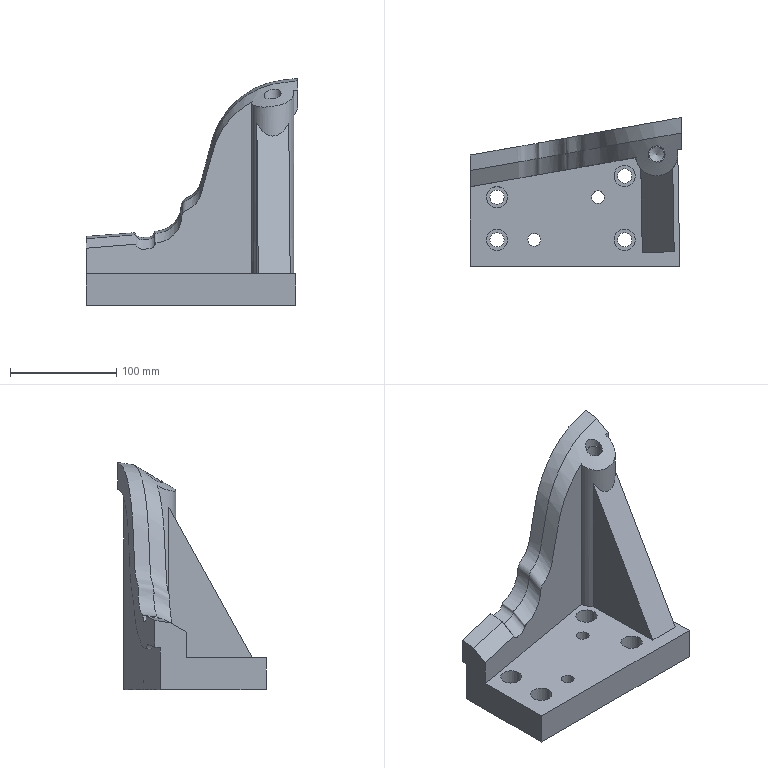Part | NX | features solid 2 | 1 solid | 39 faces | box 198.518 x 139.589 x 213.56 mm | volume 1425421 mm3 | plane 14 | cylinder 13 | spline 11 | cone 1 | commonest cylinder face diameters 13.5 x4 20 x4 12 x2 14.376 x1 16 x1 40 x1